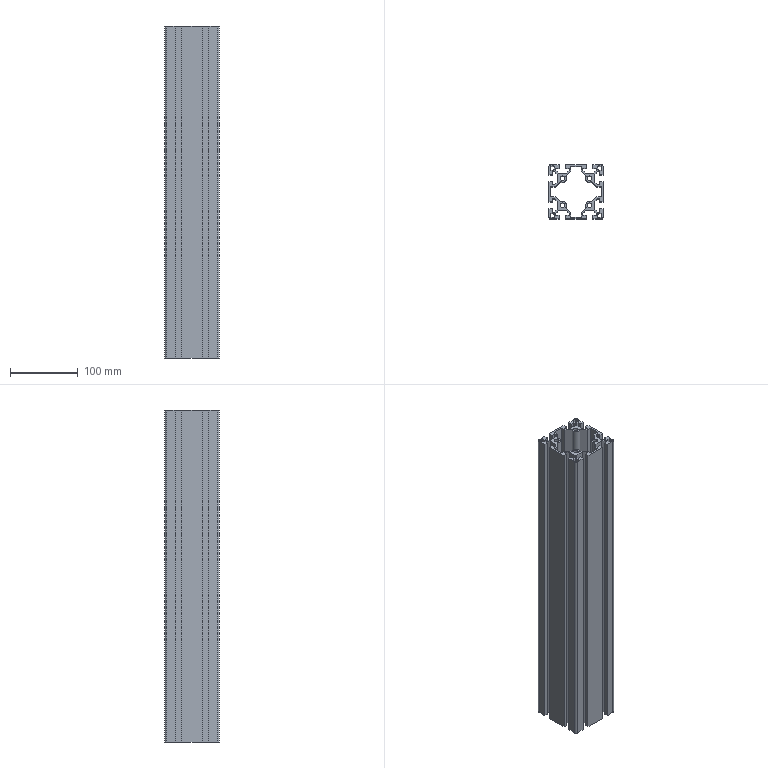Part | NX | 1 solid | 156 faces | box 80 x 80 x 490 mm | volume 858481 mm3 | plane 122 | cylinder 34 | commonest cylinder face diameters 2 x16 6.8 x8 11.8 x6 5.64 x4